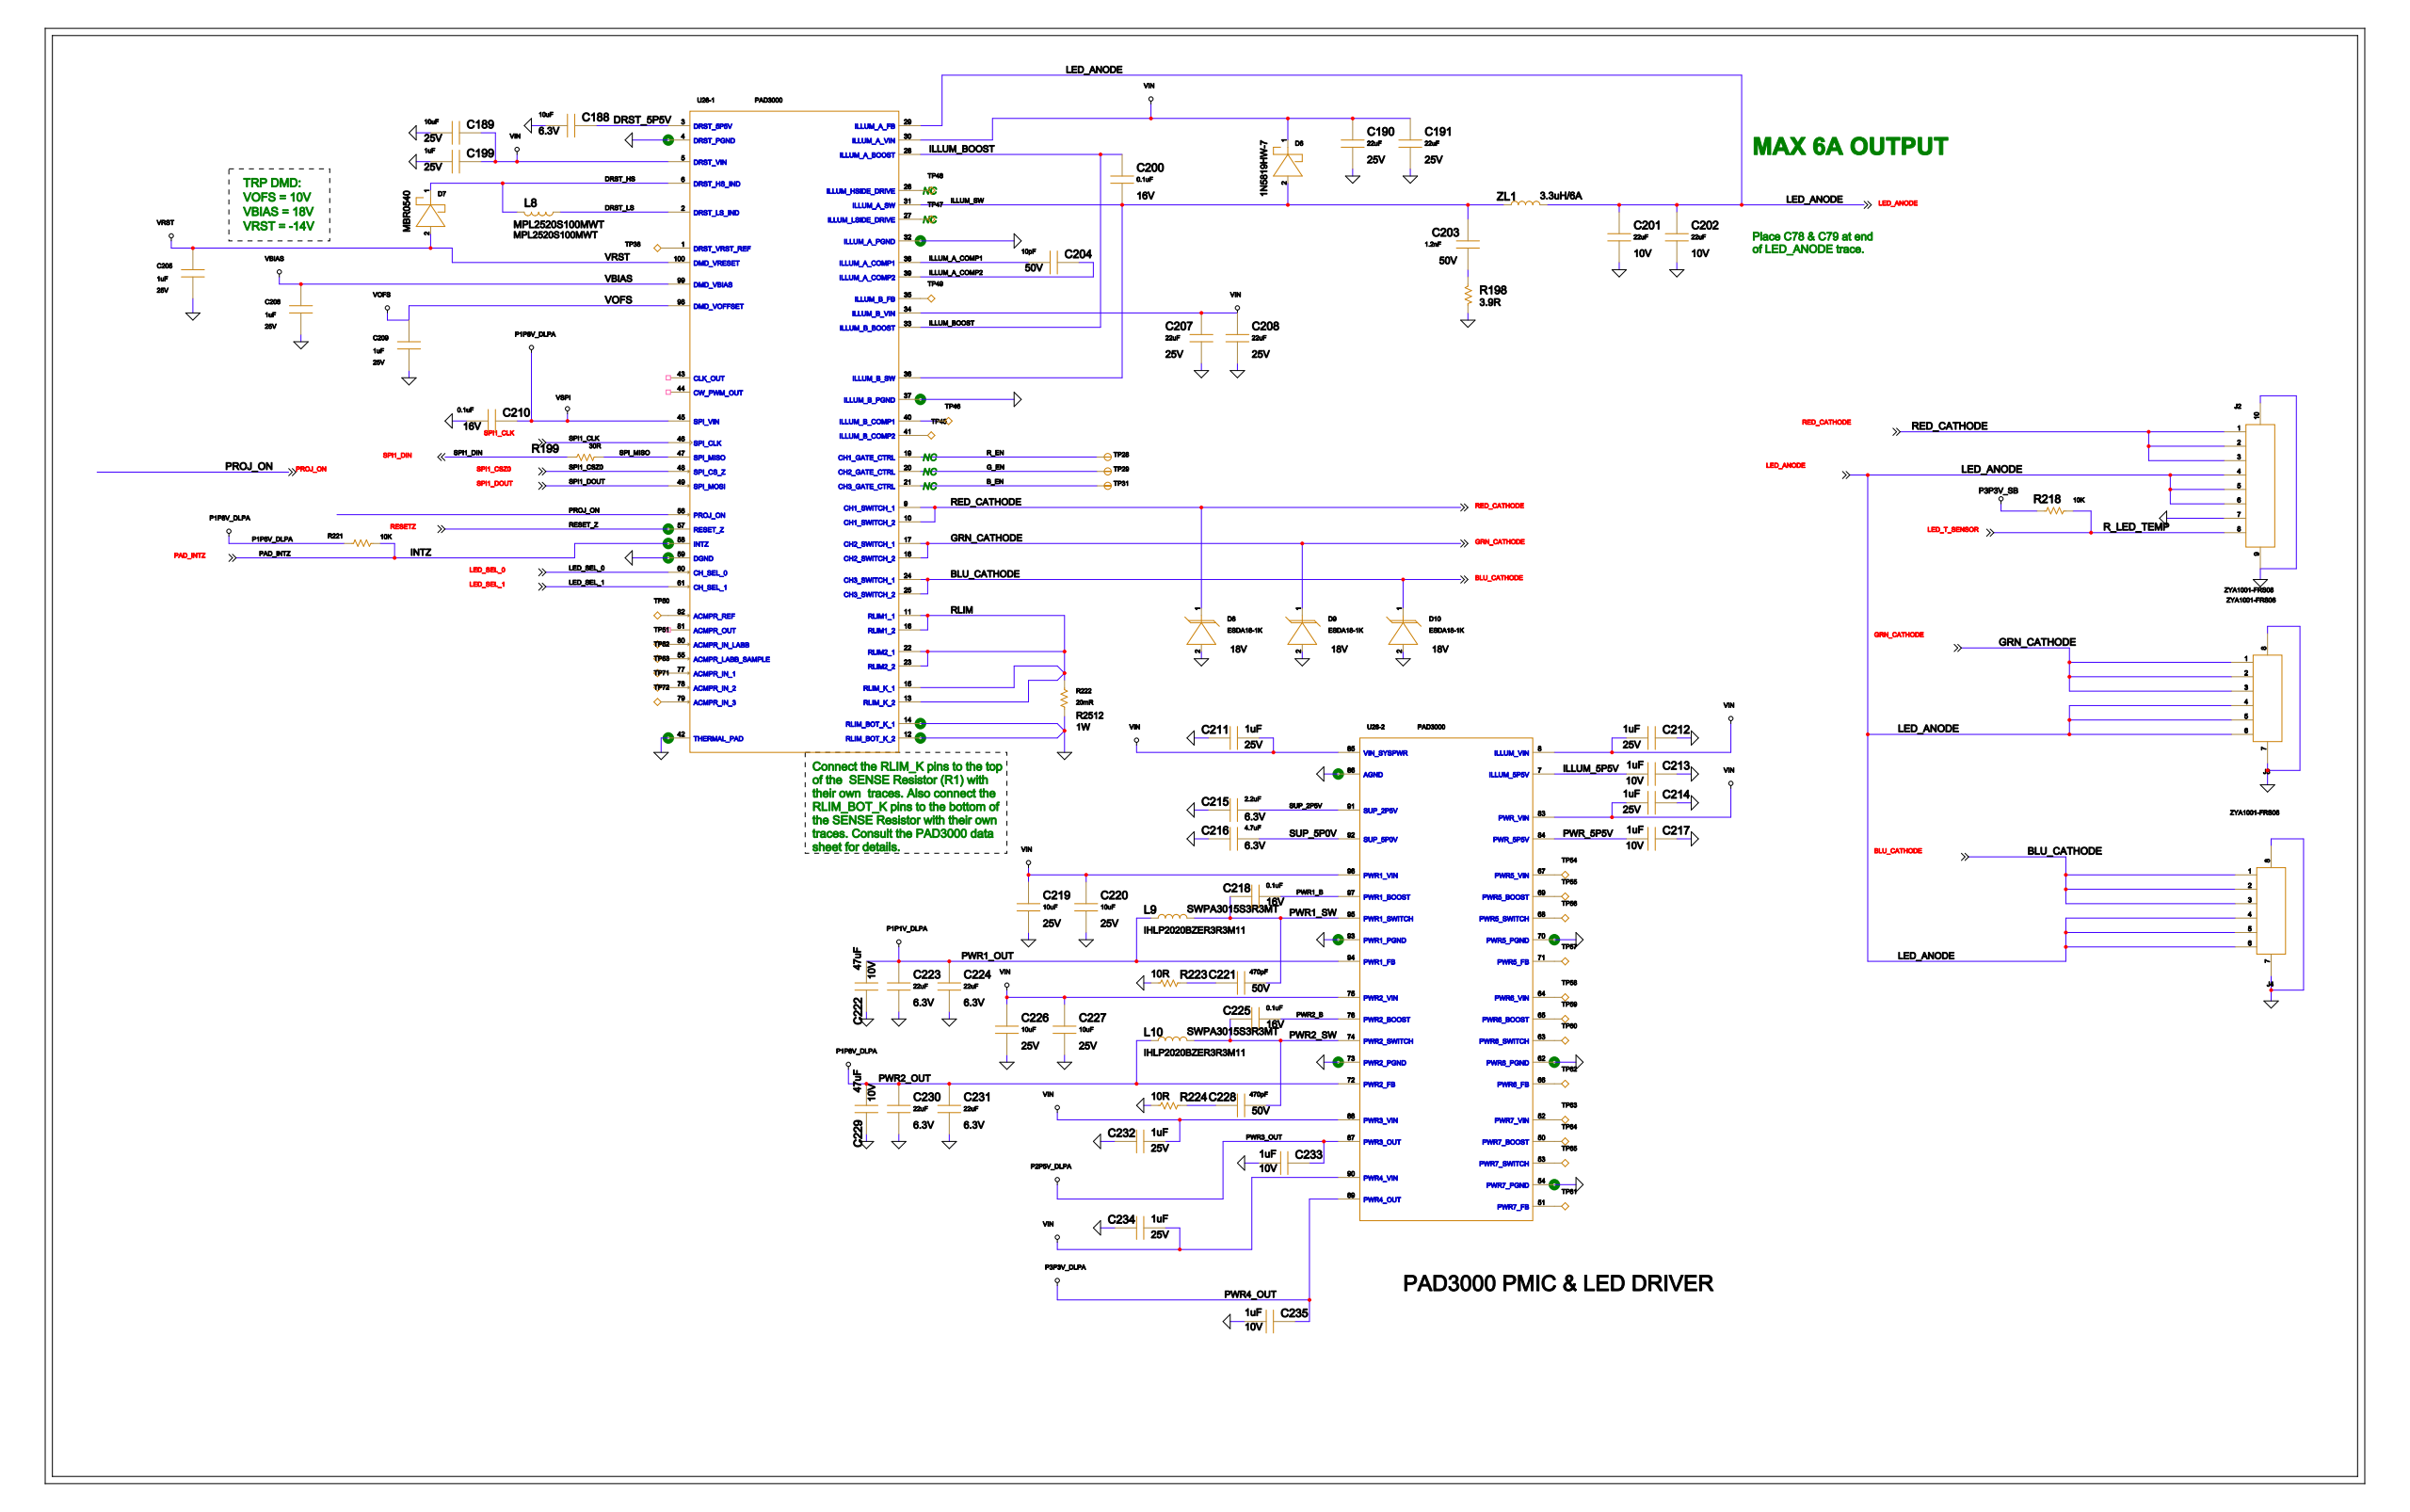Circuit board | Cadence Allegro | 1223 parts | 777 nets | one sheet of the schematic
Parts on this sheet (reference | value | footprint):
C188 | 10uF | C0603
C189 | 10uF | C0805
C190 | 22uF | C0805
C191 | 22uF | C0805
C199 | 1uF | C0402
C200 | 0.1uF | C0402
C201 | 22uF | C0805
C202 | 22uF | C0805
C203 | 1.2nF | C0603
C204 | 10pF | C0402
C205 | 1uF | C0603
C206 | 1uF | C0603
C207 | 22uF | C0805
C208 | 22uF | C0805
C209 | 1uF | C0603
C210 | 0.1uF | C0201
C211 | 1uF | C0402
C212 | 1uF | C0402
C213 | 1uF | C0402
C214 | 1uF | C0402
C215 | 2.2uF | C0402
C216 | 4.7uF | C0402
C217 | 1uF | C0402
C218 | 0.1uF | C0402
C219 | 10uF | C0805
C220 | 10uF | C0805
C221 | 470pF | C0402
C222 | 47uF | C0805
C223 | 22uF | C0603
C224 | 22uF | C0603
C225 | 0.1uF | C0402
C226 | 10uF | C0805
C227 | 10uF | C0805
C228 | 470pF | C0402
C229 | 47uF | C0805
C230 | 22uF | C0603
C231 | 22uF | C0603
C232 | 1uF | C0402
C233 | 1uF | C0402
C234 | 1uF | C0402
C235 | 1uF | C0402
D6 | 1N5819HW-7 | SOD123
D7 | MBR0540 | SOD123
D8 | ESDA18-1K | SOD523
D9 | ESDA18-1K | SOD523
D10 | ESDA18-1K | SOD523
J2 | ZYA1001-FRS08 | ZYA1001-FRS08
J3 | ZYA1001-FRS06 | ZYA1001-FRS06
J4 | ZYA1001-FRS06 | ZYA1001-FRS06
L8 | MPL2520S100MWT | 1008_2P5MMX2MM
L9 | SWPA3015S3R3MT | SMD03X03
L10 | SWPA3015S3R3MT | SMD03X03
R198 | 3.9R | R0603
R199 | 30R | R0201
R218 | 10K | R0201
R221 | 10K | R0201
R222 | 20mR | R2512
R223 | 10R | R0402
R224 | 10R | R0402
TP28 | TP40 | TP06MM
TP29 | TP40 | TP06MM
TP31 | TP40 | TP06MM
TP38 | TP40 | TP06MM
TP45 | TP40 | TP06MM
TP46 | TP40 | TP06MM
TP47 | TP40 | TP06MM
TP48 | TP40 | TP06MM
TP49 | TP40 | TP06MM
TP50 | TP40 | TP06MM
TP51 | TP40 | TP06MM
TP52 | TP40 | TP06MM
TP53 | TP40 | TP06MM
TP54 | TP40 | TP06MM
TP55 | TP40 | TP06MM
TP56 | TP40 | TP06MM
TP57 | TP40 | TP06MM
TP58 | TP40 | TP06MM
TP59 | TP40 | TP06MM
TP60 | TP40 | TP06MM
TP61 | TP40 | TP06MM
TP62 | TP40 | TP06MM
TP63 | TP40 | TP06MM
TP64 | TP40 | TP06MM
TP65 | TP40 | TP06MM
TP71 | TP40 | TP06MM
TP72 | TP40 | TP06MM
ZL1 | 3.3uH/6A | L-TMPC0603H
Nets of these parts (net: part-pin ...):
GND: C188-1 C189-2 C190-2 C191-2 C199-2 C201-2 C202-2 C205-2 C206-2 C207-2 C208-2 C209-2 C210-2 C211-2 C212-2 C213-2 C214-2 C215-1 C216-1 C217-2 C219-2 C220-2 C222-2 C223-2 C224-2 C226-2 C227-2 C229-2 C230-2 C231-2 C232-2 C233-2 C234-2 C235-2 D8-2 D9-2 D10-2 J2-7 J2-9 J2-10 J3-7 J3-8 J4-7 J4-8 R198-1 R222-1 R223-2 R224-2
P1P8V_DLPA: C210-1 C229-1 C230-1 C231-1 L10-2 R221-1
P3P3V_SB: R218-1
P1P1V_DLPA: C222-1 C223-1 C224-1 L9-2
VDLP: C189-1 C190-1 C191-1 C199-1 C207-1 C208-1 C211-1 C212-1 C214-1 C219-1 C220-1 C226-1 C227-1 C232-1 C234-1 D6-1
VBIAS: C206-1
VOFS: C209-1
VRST: C205-1 D7-2
ILLUM_SW: C200-2 C203-1 D6-2 ZL1-2
ILLUM_BOOST: C200-1
PWR1_SW: C218-2 C221-2 L9-1
PWR1_B: C218-1
PWR2_SW: C225-2 C228-2 L10-1
PWR2_B: C225-1
ILLUM_5P5V: C213-1
PWR_5P5V: C217-1
P2P5V_DLPA: C233-1
P3P3V_DLPA: C235-1
DRST_5P5V: C188-2
LED_ANODE: C201-1 C202-1 J2-4 J2-5 J2-6 J3-4 J3-5 J3-6 J4-4 J4-5 J4-6 ZL1-1
N23985520: C203-2 R198-2
ILLUM_A_COMP1: C204-2
ILLUM_A_COMP2: C204-1
SUP_2P5V: C215-2
SUP_5P0V: C216-2
N23985511: C221-1 R223-1
N23985580: C228-1 R224-1
BLU_CATHODE: D10-1 J4-1 J4-2 J4-3
RED_CATHODE: D8-1 J2-1 J2-2 J2-3
GRN_CATHODE: D9-1 J3-1 J3-2 J3-3
DRST_HS: D7-1 L8-2
PAD_INTZ: R221-2
N255439095: TP38-1
N2554390945: TP45-1
N25601087: TP46-1
N2554390935: TP47-1
N2554390933: TP48-1
N2554390939: TP49-1
N2554390922: TP50-1
N2554390924: TP51-1
N2554390925: TP52-1
N2554390926: TP53-1
N2554344417: TP54-1
N2554344420: TP55-1
N2554344418: TP56-1
N2554344416: TP57-1
N2554344422: TP58-1
N2554344424: TP59-1
N2554344425: TP60-1
N2554344430: TP61-1
N2554344423: TP62-1
N2554344428: TP63-1
N2554344429: TP64-1
N2554344427: TP65-1
N2554390927: TP71-1
N2554390928: TP72-1
LED_T_SENSOR: J2-8 R218-2
DRST_LS: L8-1
SPI_MISO: R199-1
SPI1_DIN: R199-2
RLIM: R222-2
R_EN: TP28-1
G_EN: TP29-1
B_EN: TP31-1